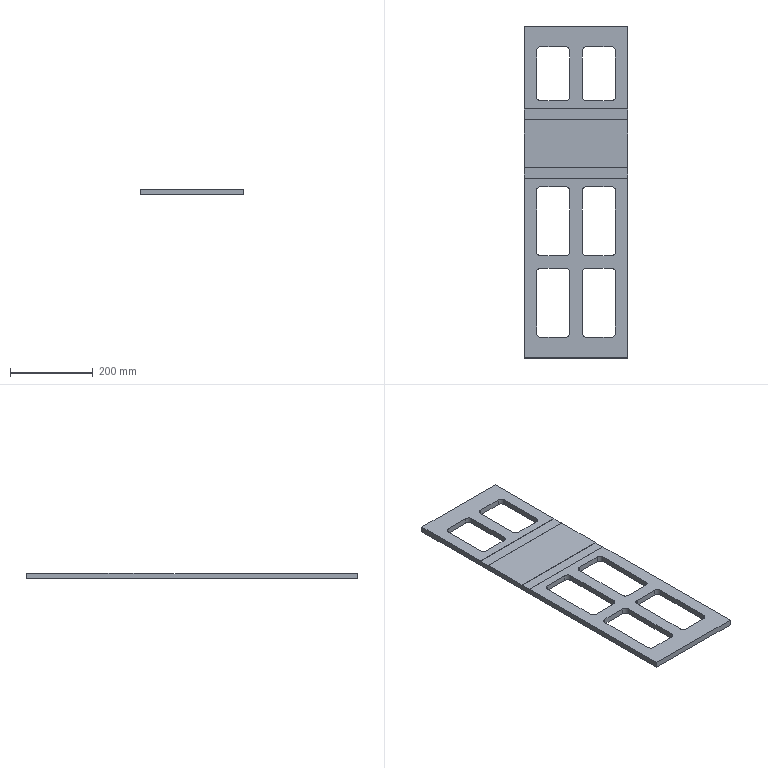Part | SolidWorks | features ICE 2, Extrusion 1, Fillet 1 | 1 solid | 62 faces | box 250 x 800 x 14 mm | volume 1757091 mm3 | plane 38 | cylinder 24 | commonest cylinder face diameters 20 x24